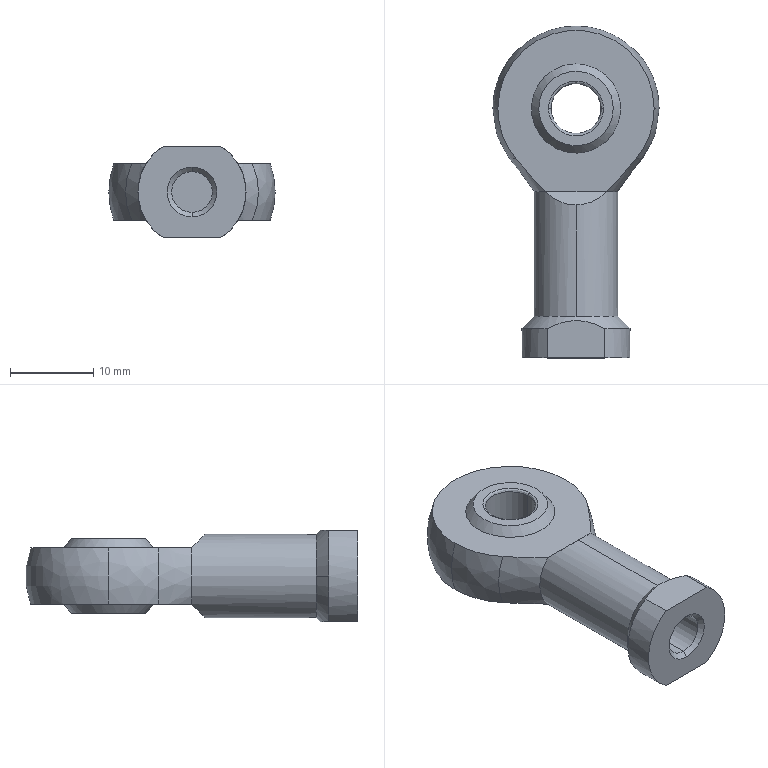Part | SolidWorks | features BaseBody 1 | 1 solid | 35 faces | box 20 x 39.987 x 11 mm | volume 3545 mm3 | plane 10 | spline 9 | cylinder 8 | cone 8 | commonest cylinder face diameters 4.917 x2 6 x2 10 x2 13 x2